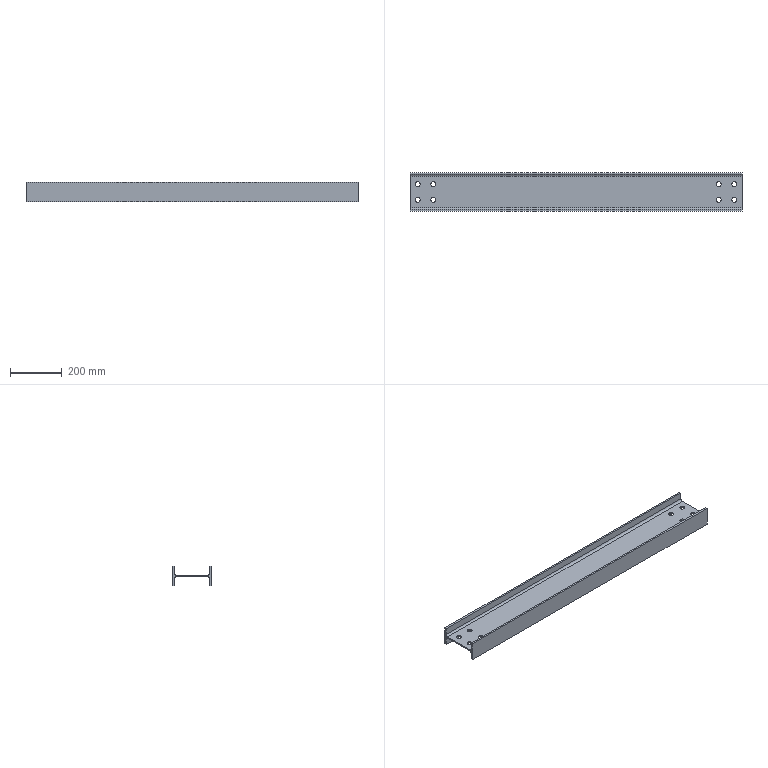Part | STEP file | 计量辅梁2_Default<As Machined> | 1 solid | 34 faces | box 1280 x 150 x 75 mm | volume 2273380 mm3 | cylinder 20 | plane 14 | commonest cylinder face diameters 19 x16 16 x4